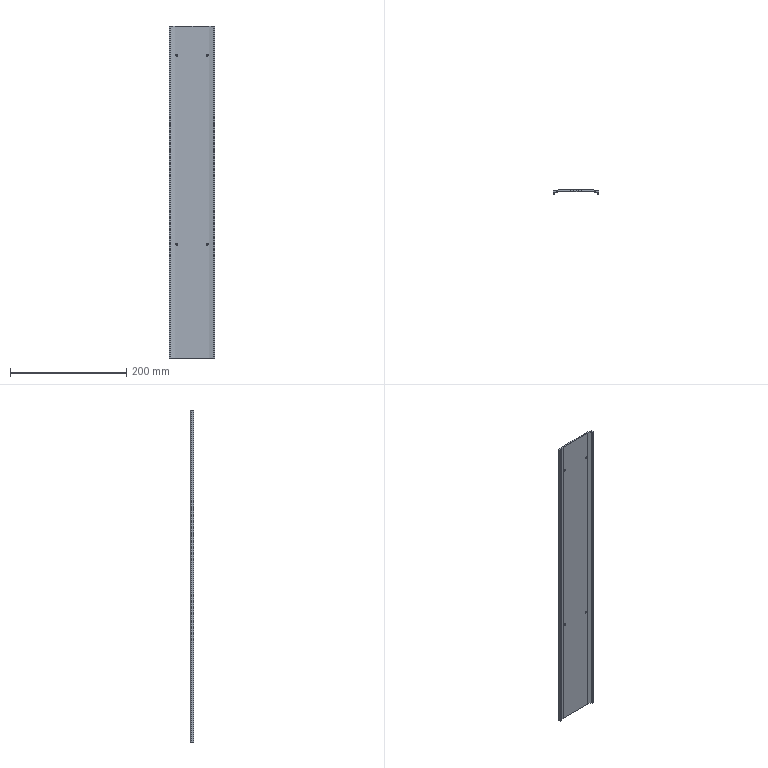Part | NX | 1 solid | 37 faces | box 79 x 6 x 572 mm | volume 116838 mm3 | plane 29 | cylinder 4 | cone 4 | commonest cylinder face diameters 3.4 x4
STEP:
#1=CARTESIAN_POINT('',(518.205,169.433,382.));
#2=VERTEX_POINT('',#1);
#3=CARTESIAN_POINT('',(518.205,165.108,382.));
#4=VERTEX_POINT('',#3);
#5=CARTESIAN_POINT('',(518.205,169.433,382.));
#6=DIRECTION('',(0.,-1.,0.));
#7=VECTOR('',#6,1.);
#8=LINE('',#5,#7);
#9=EDGE_CURVE('',#2,#4,#8,.T.);
#10=ORIENTED_EDGE('',*,*,#9,.F.);
#11=CARTESIAN_POINT('',(518.205,169.433,-190.));
#12=VERTEX_POINT('',#11);
#13=CARTESIAN_POINT('',(518.205,169.433,0.));
#14=DIRECTION('',(0.,0.,1.));
#15=VECTOR('',#14,1.);
#16=LINE('',#13,#15);
#17=EDGE_CURVE('',#12,#2,#16,.T.);
#18=ORIENTED_EDGE('',*,*,#17,.F.);
#19=CARTESIAN_POINT('',(518.205,165.108,-190.));
#20=VERTEX_POINT('',#19);
#21=CARTESIAN_POINT('',(518.205,0.,-190.));
#22=DIRECTION('',(0.,-1.,0.));
#23=VECTOR('',#22,1.);
#24=LINE('',#21,#23);
#25=EDGE_CURVE('',#12,#20,#24,.T.);
#26=ORIENTED_EDGE('',*,*,#25,.T.);
#27=CARTESIAN_POINT('',(518.205,165.108,0.));
#28=DIRECTION('',(0.,0.,1.));
#29=VECTOR('',#28,1.);
#30=LINE('',#27,#29);
#31=EDGE_CURVE('',#20,#4,#30,.T.);
#32=ORIENTED_EDGE('',*,*,#31,.T.);
#33=EDGE_LOOP('',(#10,#18,#26,#32));
#34=FACE_OUTER_BOUND('',#33,.T.);
#35=CARTESIAN_POINT('',(518.205,169.433,0.));
#36=DIRECTION('',(-1.,0.,0.));
#37=DIRECTION('',(0.,0.,-1.));
#38=AXIS2_PLACEMENT_3D('',#35,#36,#37);
#39=PLANE('',#38);
#40=ADVANCED_FACE('',(#34),#39,.T.);
#41=CARTESIAN_POINT('',(520.205,165.108,382.));
#42=VERTEX_POINT('',#41);
#43=CARTESIAN_POINT('',(518.205,165.108,382.));
#44=DIRECTION('',(1.,0.,0.));
#45=VECTOR('',#44,1.);
#46=LINE('',#43,#45);
#47=EDGE_CURVE('',#4,#42,#46,.T.);
#48=ORIENTED_EDGE('',*,*,#47,.F.);
#49=ORIENTED_EDGE('',*,*,#31,.F.);
#50=CARTESIAN_POINT('',(520.205,165.108,-190.));
#51=VERTEX_POINT('',#50);
#52=CARTESIAN_POINT('',(0.,165.108,-190.));
#53=DIRECTION('',(1.,0.,0.));
#54=VECTOR('',#53,1.);
#55=LINE('',#52,#54);
#56=EDGE_CURVE('',#20,#51,#55,.T.);
#57=ORIENTED_EDGE('',*,*,#56,.T.);
#58=CARTESIAN_POINT('',(520.205,165.108,0.));
#59=DIRECTION('',(0.,0.,1.));
#60=VECTOR('',#59,1.);
#61=LINE('',#58,#60);
#62=EDGE_CURVE('',#51,#42,#61,.T.);
#63=ORIENTED_EDGE('',*,*,#62,.T.);
#64=EDGE_LOOP('',(#48,#49,#57,#63));
#65=FACE_OUTER_BOUND('',#64,.T.);
#66=CARTESIAN_POINT('',(518.205,165.108,0.));
#67=DIRECTION('',(0.,-1.,0.));
#68=DIRECTION('',(0.,0.,1.));
#69=AXIS2_PLACEMENT_3D('',#66,#67,#68);
#70=PLANE('',#69);
#71=ADVANCED_FACE('',(#65),#70,.T.);
#72=CARTESIAN_POINT('',(520.205,167.247,382.));
#73=VERTEX_POINT('',#72);
#74=CARTESIAN_POINT('',(520.205,165.108,382.));
#75=DIRECTION('',(0.,1.,0.));
#76=VECTOR('',#75,1.);
#77=LINE('',#74,#76);
#78=EDGE_CURVE('',#42,#73,#77,.T.);
#79=ORIENTED_EDGE('',*,*,#78,.F.);
#80=ORIENTED_EDGE('',*,*,#62,.F.);
#81=CARTESIAN_POINT('',(520.205,167.247,-190.));
#82=VERTEX_POINT('',#81);
#83=CARTESIAN_POINT('',(520.205,0.,-190.));
#84=DIRECTION('',(0.,1.,0.));
#85=VECTOR('',#84,1.);
#86=LINE('',#83,#85);
#87=EDGE_CURVE('',#51,#82,#86,.T.);
#88=ORIENTED_EDGE('',*,*,#87,.T.);
#89=CARTESIAN_POINT('',(520.205,167.247,0.));
#90=DIRECTION('',(0.,0.,1.));
#91=VECTOR('',#90,1.);
#92=LINE('',#89,#91);
#93=EDGE_CURVE('',#82,#73,#92,.T.);
#94=ORIENTED_EDGE('',*,*,#93,.T.);
#95=EDGE_LOOP('',(#79,#80,#88,#94));
#96=FACE_OUTER_BOUND('',#95,.T.);
#97=CARTESIAN_POINT('',(520.205,165.108,0.));
#98=DIRECTION('',(1.,0.,0.));
#99=DIRECTION('',(0.,0.,1.));
#100=AXIS2_PLACEMENT_3D('',#97,#98,#99);
#101=PLANE('',#100);
#102=ADVANCED_FACE('',(#96),#101,.T.);
#103=CARTESIAN_POINT('',(527.924,168.608,382.));
#104=VERTEX_POINT('',#103);
#105=CARTESIAN_POINT('',(520.205,167.247,382.));
#106=DIRECTION('',(0.9848,0.1736,0.));
#107=VECTOR('',#106,1.);
#108=LINE('',#105,#107);
#109=EDGE_CURVE('',#73,#104,#108,.T.);
#110=ORIENTED_EDGE('',*,*,#109,.F.);
#111=ORIENTED_EDGE('',*,*,#93,.F.);
#112=CARTESIAN_POINT('',(527.924,168.608,-190.));
#113=VERTEX_POINT('',#112);
#114=CARTESIAN_POINT('',(-12.915,73.244,-190.));
#115=DIRECTION('',(0.9848,0.1736,0.));
#116=VECTOR('',#115,1.);
#117=LINE('',#114,#116);
#118=EDGE_CURVE('',#82,#113,#117,.T.);
#119=ORIENTED_EDGE('',*,*,#118,.T.);
#120=CARTESIAN_POINT('',(527.924,168.608,0.));
#121=DIRECTION('',(0.,0.,1.));
#122=VECTOR('',#121,1.);
#123=LINE('',#120,#122);
#124=EDGE_CURVE('',#113,#104,#123,.T.);
#125=ORIENTED_EDGE('',*,*,#124,.T.);
#126=EDGE_LOOP('',(#110,#111,#119,#125));
#127=FACE_OUTER_BOUND('',#126,.T.);
#128=CARTESIAN_POINT('',(520.205,167.247,0.));
#129=DIRECTION('',(0.1736,-0.9848,0.));
#130=DIRECTION('',(-0.9848,-0.1736,0.));
#131=AXIS2_PLACEMENT_3D('',#128,#129,#130);
#132=PLANE('',#131);
#133=ADVANCED_FACE('',(#127),#132,.T.);
#134=CARTESIAN_POINT('',(531.705,168.608,329.8));
#135=VERTEX_POINT('',#134);
#136=CARTESIAN_POINT('',(531.705,168.608,331.5));
#137=DIRECTION('',(0.,-1.,0.));
#138=DIRECTION('',(0.,0.,-1.));
#139=AXIS2_PLACEMENT_3D('',#136,#137,#138);
#140=CIRCLE('',#139,1.7);
#141=EDGE_CURVE('',#135,#135,#140,.T.);
#142=ORIENTED_EDGE('',*,*,#141,.F.);
#143=EDGE_LOOP('',(#142));
#144=FACE_BOUND('',#143,.T.);
#145=CARTESIAN_POINT('',(583.705,168.608,4.3));
#146=VERTEX_POINT('',#145);
#147=CARTESIAN_POINT('',(583.705,168.608,6.));
#148=DIRECTION('',(0.,-1.,0.));
#149=DIRECTION('',(0.,0.,-1.));
#150=AXIS2_PLACEMENT_3D('',#147,#148,#149);
#151=CIRCLE('',#150,1.7);
#152=EDGE_CURVE('',#146,#146,#151,.T.);
#153=ORIENTED_EDGE('',*,*,#152,.F.);
#154=EDGE_LOOP('',(#153));
#155=FACE_BOUND('',#154,.T.);
#156=CARTESIAN_POINT('',(583.705,168.608,329.8));
#157=VERTEX_POINT('',#156);
#158=CARTESIAN_POINT('',(583.705,168.608,331.5));
#159=DIRECTION('',(0.,-1.,0.));
#160=DIRECTION('',(0.,0.,-1.));
#161=AXIS2_PLACEMENT_3D('',#158,#159,#160);
#162=CIRCLE('',#161,1.7);
#163=EDGE_CURVE('',#157,#157,#162,.T.);
#164=ORIENTED_EDGE('',*,*,#163,.F.);
#165=EDGE_LOOP('',(#164));
#166=FACE_BOUND('',#165,.T.);
#167=CARTESIAN_POINT('',(531.705,168.608,4.3));
#168=VERTEX_POINT('',#167);
#169=CARTESIAN_POINT('',(531.705,168.608,6.));
#170=DIRECTION('',(0.,-1.,0.));
#171=DIRECTION('',(0.,0.,-1.));
#172=AXIS2_PLACEMENT_3D('',#169,#170,#171);
#173=CIRCLE('',#172,1.7);
#174=EDGE_CURVE('',#168,#168,#173,.T.);
#175=ORIENTED_EDGE('',*,*,#174,.F.);
#176=EDGE_LOOP('',(#175));
#177=FACE_BOUND('',#176,.T.);
#178=CARTESIAN_POINT('',(587.487,168.608,382.));
#179=VERTEX_POINT('',#178);
#180=CARTESIAN_POINT('',(527.924,168.608,382.));
#181=DIRECTION('',(1.,0.,0.));
#182=VECTOR('',#181,1.);
#183=LINE('',#180,#182);
#184=EDGE_CURVE('',#104,#179,#183,.T.);
#185=ORIENTED_EDGE('',*,*,#184,.F.);
#186=ORIENTED_EDGE('',*,*,#124,.F.);
#187=CARTESIAN_POINT('',(587.487,168.608,-190.));
#188=VERTEX_POINT('',#187);
#189=CARTESIAN_POINT('',(0.,168.608,-190.));
#190=DIRECTION('',(1.,0.,0.));
#191=VECTOR('',#190,1.);
#192=LINE('',#189,#191);
#193=EDGE_CURVE('',#113,#188,#192,.T.);
#194=ORIENTED_EDGE('',*,*,#193,.T.);
#195=CARTESIAN_POINT('',(587.487,168.608,0.));
#196=DIRECTION('',(0.,0.,1.));
#197=VECTOR('',#196,1.);
#198=LINE('',#195,#197);
#199=EDGE_CURVE('',#188,#179,#198,.T.);
#200=ORIENTED_EDGE('',*,*,#199,.T.);
#201=EDGE_LOOP('',(#185,#186,#194,#200));
#202=FACE_BOUND('',#201,.T.);
#203=CARTESIAN_POINT('',(527.924,168.608,0.));
#204=DIRECTION('',(0.,-1.,0.));
#205=DIRECTION('',(0.,0.,1.));
#206=AXIS2_PLACEMENT_3D('',#203,#204,#205);
#207=PLANE('',#206);
#208=ADVANCED_FACE('',(#144,#155,#166,#177,#202),#207,.T.);
#209=CARTESIAN_POINT('',(595.205,167.247,382.));
#210=VERTEX_POINT('',#209);
#211=CARTESIAN_POINT('',(587.487,168.608,382.));
#212=DIRECTION('',(0.9848,-0.1736,0.));
#213=VECTOR('',#212,1.);
#214=LINE('',#211,#213);
#215=EDGE_CURVE('',#179,#210,#214,.T.);
#216=ORIENTED_EDGE('',*,*,#215,.F.);
#217=ORIENTED_EDGE('',*,*,#199,.F.);
#218=CARTESIAN_POINT('',(595.205,167.247,-190.));
#219=VERTEX_POINT('',#218);
#220=CARTESIAN_POINT('',(46.549,263.99,-190.));
#221=DIRECTION('',(0.9848,-0.1736,0.));
#222=VECTOR('',#221,1.);
#223=LINE('',#220,#222);
#224=EDGE_CURVE('',#188,#219,#223,.T.);
#225=ORIENTED_EDGE('',*,*,#224,.T.);
#226=CARTESIAN_POINT('',(595.205,167.247,0.));
#227=DIRECTION('',(0.,0.,1.));
#228=VECTOR('',#227,1.);
#229=LINE('',#226,#228);
#230=EDGE_CURVE('',#219,#210,#229,.T.);
#231=ORIENTED_EDGE('',*,*,#230,.T.);
#232=EDGE_LOOP('',(#216,#217,#225,#231));
#233=FACE_OUTER_BOUND('',#232,.T.);
#234=CARTESIAN_POINT('',(587.487,168.608,0.));
#235=DIRECTION('',(-0.1736,-0.9848,0.));
#236=DIRECTION('',(-0.9848,0.1736,0.));
#237=AXIS2_PLACEMENT_3D('',#234,#235,#236);
#238=PLANE('',#237);
#239=ADVANCED_FACE('',(#233),#238,.T.);
#240=CARTESIAN_POINT('',(595.205,165.108,382.));
#241=VERTEX_POINT('',#240);
#242=CARTESIAN_POINT('',(595.205,167.247,382.));
#243=DIRECTION('',(0.,-1.,0.));
#244=VECTOR('',#243,1.);
#245=LINE('',#242,#244);
#246=EDGE_CURVE('',#210,#241,#245,.T.);
#247=ORIENTED_EDGE('',*,*,#246,.F.);
#248=ORIENTED_EDGE('',*,*,#230,.F.);
#249=CARTESIAN_POINT('',(595.205,165.108,-190.));
#250=VERTEX_POINT('',#249);
#251=CARTESIAN_POINT('',(595.205,0.,-190.));
#252=DIRECTION('',(0.,-1.,0.));
#253=VECTOR('',#252,1.);
#254=LINE('',#251,#253);
#255=EDGE_CURVE('',#219,#250,#254,.T.);
#256=ORIENTED_EDGE('',*,*,#255,.T.);
#257=CARTESIAN_POINT('',(595.205,165.108,0.));
#258=DIRECTION('',(0.,0.,1.));
#259=VECTOR('',#258,1.);
#260=LINE('',#257,#259);
#261=EDGE_CURVE('',#250,#241,#260,.T.);
#262=ORIENTED_EDGE('',*,*,#261,.T.);
#263=EDGE_LOOP('',(#247,#248,#256,#262));
#264=FACE_OUTER_BOUND('',#263,.T.);
#265=CARTESIAN_POINT('',(595.205,167.247,0.));
#266=DIRECTION('',(-1.,0.,0.));
#267=DIRECTION('',(0.,0.,-1.));
#268=AXIS2_PLACEMENT_3D('',#265,#266,#267);
#269=PLANE('',#268);
#270=ADVANCED_FACE('',(#264),#269,.T.);
#271=CARTESIAN_POINT('',(597.205,165.108,382.));
#272=VERTEX_POINT('',#271);
#273=CARTESIAN_POINT('',(595.205,165.108,382.));
#274=DIRECTION('',(1.,0.,0.));
#275=VECTOR('',#274,1.);
#276=LINE('',#273,#275);
#277=EDGE_CURVE('',#241,#272,#276,.T.);
#278=ORIENTED_EDGE('',*,*,#277,.F.);
#279=ORIENTED_EDGE('',*,*,#261,.F.);
#280=CARTESIAN_POINT('',(597.205,165.108,-190.));
#281=VERTEX_POINT('',#280);
#282=CARTESIAN_POINT('',(0.,165.108,-190.));
#283=DIRECTION('',(1.,0.,0.));
#284=VECTOR('',#283,1.);
#285=LINE('',#282,#284);
#286=EDGE_CURVE('',#250,#281,#285,.T.);
#287=ORIENTED_EDGE('',*,*,#286,.T.);
#288=CARTESIAN_POINT('',(597.205,165.108,0.));
#289=DIRECTION('',(0.,0.,1.));
#290=VECTOR('',#289,1.);
#291=LINE('',#288,#290);
#292=EDGE_CURVE('',#281,#272,#291,.T.);
#293=ORIENTED_EDGE('',*,*,#292,.T.);
#294=EDGE_LOOP('',(#278,#279,#287,#293));
#295=FACE_OUTER_BOUND('',#294,.T.);
#296=CARTESIAN_POINT('',(595.205,165.108,0.));
#297=DIRECTION('',(0.,-1.,0.));
#298=DIRECTION('',(0.,0.,1.));
#299=AXIS2_PLACEMENT_3D('',#296,#297,#298);
#300=PLANE('',#299);
#301=ADVANCED_FACE('',(#295),#300,.T.);
#302=CARTESIAN_POINT('',(597.205,169.433,382.));
#303=VERTEX_POINT('',#302);
#304=CARTESIAN_POINT('',(597.205,165.108,382.));
#305=DIRECTION('',(0.,1.,0.));
#306=VECTOR('',#305,1.);
#307=LINE('',#304,#306);
#308=EDGE_CURVE('',#272,#303,#307,.T.);
#309=ORIENTED_EDGE('',*,*,#308,.F.);
#310=ORIENTED_EDGE('',*,*,#292,.F.);
#311=CARTESIAN_POINT('',(597.205,169.433,-190.));
#312=VERTEX_POINT('',#311);
#313=CARTESIAN_POINT('',(597.205,0.,-190.));
#314=DIRECTION('',(0.,1.,0.));
#315=VECTOR('',#314,1.);
#316=LINE('',#313,#315);
#317=EDGE_CURVE('',#281,#312,#316,.T.);
#318=ORIENTED_EDGE('',*,*,#317,.T.);
#319=CARTESIAN_POINT('',(597.205,169.433,0.));
#320=DIRECTION('',(0.,0.,1.));
#321=VECTOR('',#320,1.);
#322=LINE('',#319,#321);
#323=EDGE_CURVE('',#312,#303,#322,.T.);
#324=ORIENTED_EDGE('',*,*,#323,.T.);
#325=EDGE_LOOP('',(#309,#310,#318,#324));
#326=FACE_OUTER_BOUND('',#325,.T.);
#327=CARTESIAN_POINT('',(597.205,165.108,0.));
#328=DIRECTION('',(1.,0.,0.));
#329=DIRECTION('',(0.,0.,1.));
#330=AXIS2_PLACEMENT_3D('',#327,#328,#329);
#331=PLANE('',#330);
#332=ADVANCED_FACE('',(#326),#331,.T.);
#333=CARTESIAN_POINT('',(587.705,171.108,382.));
#334=VERTEX_POINT('',#333);
#335=CARTESIAN_POINT('',(597.205,169.433,382.));
#336=DIRECTION('',(-0.9848,0.1736,0.));
#337=VECTOR('',#336,1.);
#338=LINE('',#335,#337);
#339=EDGE_CURVE('',#303,#334,#338,.T.);
#340=ORIENTED_EDGE('',*,*,#339,.F.);
#341=ORIENTED_EDGE('',*,*,#323,.F.);
#342=CARTESIAN_POINT('',(587.705,171.108,-190.));
#343=VERTEX_POINT('',#342);
#344=CARTESIAN_POINT('',(46.983,266.452,-190.));
#345=DIRECTION('',(-0.9848,0.1736,0.));
#346=VECTOR('',#345,1.);
#347=LINE('',#344,#346);
#348=EDGE_CURVE('',#312,#343,#347,.T.);
#349=ORIENTED_EDGE('',*,*,#348,.T.);
#350=CARTESIAN_POINT('',(587.705,171.108,0.));
#351=DIRECTION('',(0.,0.,1.));
#352=VECTOR('',#351,1.);
#353=LINE('',#350,#352);
#354=EDGE_CURVE('',#343,#334,#353,.T.);
#355=ORIENTED_EDGE('',*,*,#354,.T.);
#356=EDGE_LOOP('',(#340,#341,#349,#355));
#357=FACE_OUTER_BOUND('',#356,.T.);
#358=CARTESIAN_POINT('',(597.205,169.433,0.));
#359=DIRECTION('',(0.1736,0.9848,0.));
#360=DIRECTION('',(0.9848,-0.1736,0.));
#361=AXIS2_PLACEMENT_3D('',#358,#359,#360);
#362=PLANE('',#361);
#363=ADVANCED_FACE('',(#357),#362,.T.);
#364=CARTESIAN_POINT('',(583.705,171.108,9.3));
#365=VERTEX_POINT('',#364);
#366=CARTESIAN_POINT('',(583.705,171.108,6.));
#367=DIRECTION('',(0.,-1.,0.));
#368=DIRECTION('',(0.,0.,1.));
#369=AXIS2_PLACEMENT_3D('',#366,#367,#368);
#370=CIRCLE('',#369,3.3);
#371=EDGE_CURVE('',#365,#365,#370,.T.);
#372=ORIENTED_EDGE('',*,*,#371,.T.);
#373=EDGE_LOOP('',(#372));
#374=FACE_BOUND('',#373,.T.);
#375=CARTESIAN_POINT('',(583.705,171.108,334.8));
#376=VERTEX_POINT('',#375);
#377=CARTESIAN_POINT('',(583.705,171.108,331.5));
#378=DIRECTION('',(0.,-1.,0.));
#379=DIRECTION('',(0.,0.,1.));
#380=AXIS2_PLACEMENT_3D('',#377,#378,#379);
#381=CIRCLE('',#380,3.3);
#382=EDGE_CURVE('',#376,#376,#381,.T.);
#383=ORIENTED_EDGE('',*,*,#382,.T.);
#384=EDGE_LOOP('',(#383));
#385=FACE_BOUND('',#384,.T.);
#386=CARTESIAN_POINT('',(568.323,171.108,382.));
#387=VERTEX_POINT('',#386);
#388=CARTESIAN_POINT('',(587.705,171.108,382.));
#389=DIRECTION('',(-1.,0.,0.));
#390=VECTOR('',#389,1.);
#391=LINE('',#388,#390);
#392=EDGE_CURVE('',#334,#387,#391,.T.);
#393=ORIENTED_EDGE('',*,*,#392,.F.);
#394=ORIENTED_EDGE('',*,*,#354,.F.);
#395=CARTESIAN_POINT('',(568.323,171.108,-190.));
#396=VERTEX_POINT('',#395);
#397=CARTESIAN_POINT('',(0.,171.108,-190.));
#398=DIRECTION('',(-1.,0.,0.));
#399=VECTOR('',#398,1.);
#400=LINE('',#397,#399);
#401=EDGE_CURVE('',#343,#396,#400,.T.);
#402=ORIENTED_EDGE('',*,*,#401,.T.);
#403=CARTESIAN_POINT('',(568.323,171.108,0.));
#404=DIRECTION('',(0.,0.,1.));
#405=VECTOR('',#404,1.);
#406=LINE('',#403,#405);
#407=EDGE_CURVE('',#396,#387,#406,.T.);
#408=ORIENTED_EDGE('',*,*,#407,.T.);
#409=EDGE_LOOP('',(#393,#394,#402,#408));
#410=FACE_BOUND('',#409,.T.);
#411=CARTESIAN_POINT('',(587.705,171.108,0.));
#412=DIRECTION('',(0.,1.,0.));
#413=DIRECTION('',(0.,0.,-1.));
#414=AXIS2_PLACEMENT_3D('',#411,#412,#413);
#415=PLANE('',#414);
#416=ADVANCED_FACE('',(#374,#385,#410),#415,.T.);
#417=CARTESIAN_POINT('',(567.705,170.608,382.));
#418=VERTEX_POINT('',#417);
#419=CARTESIAN_POINT('',(568.323,171.108,382.));
#420=DIRECTION('',(-0.7774,-0.629,0.));
#421=VECTOR('',#420,1.);
#422=LINE('',#419,#421);
#423=EDGE_CURVE('',#387,#418,#422,.T.);
#424=ORIENTED_EDGE('',*,*,#423,.F.);
#425=ORIENTED_EDGE('',*,*,#407,.F.);
#426=CARTESIAN_POINT('',(567.705,170.608,-190.));
#427=VERTEX_POINT('',#426);
#428=CARTESIAN_POINT('',(141.154,-174.477,-190.));
#429=DIRECTION('',(-0.7774,-0.629,0.));
#430=VECTOR('',#429,1.);
#431=LINE('',#428,#430);
#432=EDGE_CURVE('',#396,#427,#431,.T.);
#433=ORIENTED_EDGE('',*,*,#432,.T.);
#434=CARTESIAN_POINT('',(567.705,170.608,0.));
#435=DIRECTION('',(0.,0.,1.));
#436=VECTOR('',#435,1.);
#437=LINE('',#434,#436);
#438=EDGE_CURVE('',#427,#418,#437,.T.);
#439=ORIENTED_EDGE('',*,*,#438,.T.);
#440=EDGE_LOOP('',(#424,#425,#433,#439));
#441=FACE_OUTER_BOUND('',#440,.T.);
#442=CARTESIAN_POINT('',(568.323,171.108,0.));
#443=DIRECTION('',(-0.629,0.7774,0.));
#444=DIRECTION('',(0.7774,0.629,0.));
#445=AXIS2_PLACEMENT_3D('',#442,#443,#444);
#446=PLANE('',#445);
#447=ADVANCED_FACE('',(#441),#446,.T.);
#448=CARTESIAN_POINT('',(567.087,171.108,382.));
#449=VERTEX_POINT('',#448);
#450=CARTESIAN_POINT('',(567.705,170.608,382.));
#451=DIRECTION('',(-0.7774,0.629,0.));
#452=VECTOR('',#451,1.);
#453=LINE('',#450,#452);
#454=EDGE_CURVE('',#418,#449,#453,.T.);
#455=ORIENTED_EDGE('',*,*,#454,.F.);
#456=ORIENTED_EDGE('',*,*,#438,.F.);
#457=CARTESIAN_POINT('',(567.087,171.108,-190.));
#458=VERTEX_POINT('',#457);
#459=CARTESIAN_POINT('',(308.001,380.712,-190.));
#460=DIRECTION('',(-0.7774,0.629,0.));
#461=VECTOR('',#460,1.);
#462=LINE('',#459,#461);
#463=EDGE_CURVE('',#427,#458,#462,.T.);
#464=ORIENTED_EDGE('',*,*,#463,.T.);
#465=CARTESIAN_POINT('',(567.087,171.108,0.));
#466=DIRECTION('',(0.,0.,1.));
#467=VECTOR('',#466,1.);
#468=LINE('',#465,#467);
#469=EDGE_CURVE('',#458,#449,#468,.T.);
#470=ORIENTED_EDGE('',*,*,#469,.T.);
#471=EDGE_LOOP('',(#455,#456,#464,#470));
#472=FACE_OUTER_BOUND('',#471,.T.);
#473=CARTESIAN_POINT('',(567.705,170.608,0.));
#474=DIRECTION('',(0.629,0.7774,0.));
#475=DIRECTION('',(0.7774,-0.629,0.));
#476=AXIS2_PLACEMENT_3D('',#473,#474,#475);
#477=PLANE('',#476);
#478=ADVANCED_FACE('',(#472),#477,.T.);
#479=CARTESIAN_POINT('',(563.323,171.108,382.));
#480=VERTEX_POINT('',#479);
#481=CARTESIAN_POINT('',(567.087,171.108,382.));
#482=DIRECTION('',(-1.,0.,0.));
#483=VECTOR('',#482,1.);
#484=LINE('',#481,#483);
#485=EDGE_CURVE('',#449,#480,#484,.T.);
#486=ORIENTED_EDGE('',*,*,#485,.F.);
#487=ORIENTED_EDGE('',*,*,#469,.F.);
#488=CARTESIAN_POINT('',(563.323,171.108,-190.));
#489=VERTEX_POINT('',#488);
#490=CARTESIAN_POINT('',(0.,171.108,-190.));
#491=DIRECTION('',(-1.,0.,0.));
#492=VECTOR('',#491,1.);
#493=LINE('',#490,#492);
#494=EDGE_CURVE('',#458,#489,#493,.T.);
#495=ORIENTED_EDGE('',*,*,#494,.T.);
#496=CARTESIAN_POINT('',(563.323,171.108,0.));
#497=DIRECTION('',(0.,0.,1.));
#498=VECTOR('',#497,1.);
#499=LINE('',#496,#498);
#500=EDGE_CURVE('',#489,#480,#499,.T.);
#501=ORIENTED_EDGE('',*,*,#500,.T.);
#502=EDGE_LOOP('',(#486,#487,#495,#501));
#503=FACE_OUTER_BOUND('',#502,.T.);
#504=CARTESIAN_POINT('',(567.087,171.108,0.));
#505=DIRECTION('',(0.,1.,0.));
#506=DIRECTION('',(0.,0.,-1.));
#507=AXIS2_PLACEMENT_3D('',#504,#505,#506);
#508=PLANE('',#507);
#509=ADVANCED_FACE('',(#503),#508,.T.);
#510=CARTESIAN_POINT('',(562.705,170.608,382.));
#511=VERTEX_POINT('',#510);
#512=CARTESIAN_POINT('',(563.323,171.108,382.));
#513=DIRECTION('',(-0.7774,-0.629,0.));
#514=VECTOR('',#513,1.);
#515=LINE('',#512,#514);
#516=EDGE_CURVE('',#480,#511,#515,.T.);
#517=ORIENTED_EDGE('',*,*,#516,.F.);
#518=ORIENTED_EDGE('',*,*,#500,.F.);
#519=CARTESIAN_POINT('',(562.705,170.608,-190.));
#520=VERTEX_POINT('',#519);
#521=CARTESIAN_POINT('',(139.176,-172.032,-190.));
#522=DIRECTION('',(-0.7774,-0.629,0.));
#523=VECTOR('',#522,1.);
#524=LINE('',#521,#523);
#525=EDGE_CURVE('',#489,#520,#524,.T.);
#526=ORIENTED_EDGE('',*,*,#525,.T.);
#527=CARTESIAN_POINT('',(562.705,170.608,0.));
#528=DIRECTION('',(0.,0.,1.));
#529=VECTOR('',#528,1.);
#530=LINE('',#527,#529);
#531=EDGE_CURVE('',#520,#511,#530,.T.);
#532=ORIENTED_EDGE('',*,*,#531,.T.);
#533=EDGE_LOOP('',(#517,#518,#526,#532));
#534=FACE_OUTER_BOUND('',#533,.T.);
#535=CARTESIAN_POINT('',(563.323,171.108,0.));
#536=DIRECTION('',(-0.629,0.7774,0.));
#537=DIRECTION('',(0.7774,0.629,0.));
#538=AXIS2_PLACEMENT_3D('',#535,#536,#537);
#539=PLANE('',#538);
#540=ADVANCED_FACE('',(#534),#539,.T.);
#541=CARTESIAN_POINT('',(562.087,171.108,382.));
#542=VERTEX_POINT('',#541);
#543=CARTESIAN_POINT('',(562.705,170.608,382.));
#544=DIRECTION('',(-0.7774,0.629,0.));
#545=VECTOR('',#544,1.);
#546=LINE('',#543,#545);
#547=EDGE_CURVE('',#511,#542,#546,.T.);
#548=ORIENTED_EDGE('',*,*,#547,.F.);
#549=ORIENTED_EDGE('',*,*,#531,.F.);
#550=CARTESIAN_POINT('',(562.087,171.108,-190.));
#551=VERTEX_POINT('',#550);
#552=CARTESIAN_POINT('',(306.023,378.267,-190.));
#553=DIRECTION('',(-0.7774,0.629,0.));
#554=VECTOR('',#553,1.);
#555=LINE('',#552,#554);
#556=EDGE_CURVE('',#520,#551,#555,.T.);
#557=ORIENTED_EDGE('',*,*,#556,.T.);
#558=CARTESIAN_POINT('',(562.087,171.108,0.));
#559=DIRECTION('',(0.,0.,1.));
#560=VECTOR('',#559,1.);
#561=LINE('',#558,#560);
#562=EDGE_CURVE('',#551,#542,#561,.T.);
#563=ORIENTED_EDGE('',*,*,#562,.T.);
#564=EDGE_LOOP('',(#548,#549,#557,#563));
#565=FACE_OUTER_BOUND('',#564,.T.);
#566=CARTESIAN_POINT('',(562.705,170.608,0.));
#567=DIRECTION('',(0.629,0.7774,0.));
#568=DIRECTION('',(0.7774,-0.629,0.));
#569=AXIS2_PLACEMENT_3D('',#566,#567,#568);
#570=PLANE('',#569);
#571=ADVANCED_FACE('',(#565),#570,.T.);
#572=CARTESIAN_POINT('',(558.323,171.108,382.));
#573=VERTEX_POINT('',#572);
#574=CARTESIAN_POINT('',(562.087,171.108,382.));
#575=DIRECTION('',(-1.,0.,0.));
#576=VECTOR('',#575,1.);
#577=LINE('',#574,#576);
#578=EDGE_CURVE('',#542,#573,#577,.T.);
#579=ORIENTED_EDGE('',*,*,#578,.F.);
#580=ORIENTED_EDGE('',*,*,#562,.F.);
#581=CARTESIAN_POINT('',(558.323,171.108,-190.));
#582=VERTEX_POINT('',#581);
#583=CARTESIAN_POINT('',(0.,171.108,-190.));
#584=DIRECTION('',(-1.,0.,0.));
#585=VECTOR('',#584,1.);
#586=LINE('',#583,#585);
#587=EDGE_CURVE('',#551,#582,#586,.T.);
#588=ORIENTED_EDGE('',*,*,#587,.T.);
#589=CARTESIAN_POINT('',(558.323,171.108,0.));
#590=DIRECTION('',(0.,0.,1.));
#591=VECTOR('',#590,1.);
#592=LINE('',#589,#591);
#593=EDGE_CURVE('',#582,#573,#592,.T.);
#594=ORIENTED_EDGE('',*,*,#593,.T.);
#595=EDGE_LOOP('',(#579,#580,#588,#594));
#596=FACE_OUTER_BOUND('',#595,.T.);
#597=CARTESIAN_POINT('',(562.087,171.108,0.));
#598=DIRECTION('',(0.,1.,0.));
#599=DIRECTION('',(0.,0.,-1.));
#600=AXIS2_PLACEMENT_3D('',#597,#598,#599);
#601=PLANE('',#600);
#602=ADVANCED_FACE('',(#596),#601,.T.);
#603=CARTESIAN_POINT('',(557.705,170.608,382.));
#604=VERTEX_POINT('',#603);
#605=CARTESIAN_POINT('',(558.323,171.108,382.));
#606=DIRECTION('',(-0.7774,-0.629,0.));
#607=VECTOR('',#606,1.);
#608=LINE('',#605,#607);
#609=EDGE_CURVE('',#573,#604,#608,.T.);
#610=ORIENTED_EDGE('',*,*,#609,.F.);
#611=ORIENTED_EDGE('',*,*,#593,.F.);
#612=CARTESIAN_POINT('',(557.705,170.608,-190.));
#613=VERTEX_POINT('',#612);
#614=CARTESIAN_POINT('',(137.199,-169.588,-190.));
#615=DIRECTION('',(-0.7774,-0.629,0.));
#616=VECTOR('',#615,1.);
#617=LINE('',#614,#616);
#618=EDGE_CURVE('',#582,#613,#617,.T.);
#619=ORIENTED_EDGE('',*,*,#618,.T.);
#620=CARTESIAN_POINT('',(557.705,170.608,0.));
#621=DIRECTION('',(0.,0.,1.));
#622=VECTOR('',#621,1.);
#623=LINE('',#620,#622);
#624=EDGE_CURVE('',#613,#604,#623,.T.);
#625=ORIENTED_EDGE('',*,*,#624,.T.);
#626=EDGE_LOOP('',(#610,#611,#619,#625));
#627=FACE_OUTER_BOUND('',#626,.T.);
#628=CARTESIAN_POINT('',(558.323,171.108,0.));
#629=DIRECTION('',(-0.629,0.7774,0.));
#630=DIRECTION('',(0.7774,0.629,0.));
#631=AXIS2_PLACEMENT_3D('',#628,#629,#630);
#632=PLANE('',#631);
#633=ADVANCED_FACE('',(#627),#632,.T.);
#634=CARTESIAN_POINT('',(557.087,171.108,382.));
#635=VERTEX_POINT('',#634);
#636=CARTESIAN_POINT('',(557.705,170.608,382.));
#637=DIRECTION('',(-0.7774,0.629,0.));
#638=VECTOR('',#637,1.);
#639=LINE('',#636,#638);
#640=EDGE_CURVE('',#604,#635,#639,.T.);
#641=ORIENTED_EDGE('',*,*,#640,.F.);
#642=ORIENTED_EDGE('',*,*,#624,.F.);
#643=CARTESIAN_POINT('',(557.087,171.108,-190.));
#644=VERTEX_POINT('',#643);
#645=CARTESIAN_POINT('',(304.045,375.822,-190.));
#646=DIRECTION('',(-0.7774,0.629,0.));
#647=VECTOR('',#646,1.);
#648=LINE('',#645,#647);
#649=EDGE_CURVE('',#613,#644,#648,.T.);
#650=ORIENTED_EDGE('',*,*,#649,.T.);
#651=CARTESIAN_POINT('',(557.087,171.108,0.));
#652=DIRECTION('',(0.,0.,1.));
#653=VECTOR('',#652,1.);
#654=LINE('',#651,#653);
#655=EDGE_CURVE('',#644,#635,#654,.T.);
#656=ORIENTED_EDGE('',*,*,#655,.T.);
#657=EDGE_LOOP('',(#641,#642,#650,#656));
#658=FACE_OUTER_BOUND('',#657,.T.);
#659=CARTESIAN_POINT('',(557.705,170.608,0.));
#660=DIRECTION('',(0.629,0.7774,0.));
#661=DIRECTION('',(0.7774,-0.629,0.));
#662=AXIS2_PLACEMENT_3D('',#659,#660,#661);
#663=PLANE('',#662);
#664=ADVANCED_FACE('',(#658),#663,.T.);
#665=CARTESIAN_POINT('',(553.323,171.108,382.));
#666=VERTEX_POINT('',#665);
#667=CARTESIAN_POINT('',(557.087,171.108,382.));
#668=DIRECTION('',(-1.,0.,0.));
#669=VECTOR('',#668,1.);
#670=LINE('',#667,#669);
#671=EDGE_CURVE('',#635,#666,#670,.T.);
#672=ORIENTED_EDGE('',*,*,#671,.F.);
#673=ORIENTED_EDGE('',*,*,#655,.F.);
#674=CARTESIAN_POINT('',(553.323,171.108,-190.));
#675=VERTEX_POINT('',#674);
#676=CARTESIAN_POINT('',(0.,171.108,-190.));
#677=DIRECTION('',(-1.,0.,0.));
#678=VECTOR('',#677,1.);
#679=LINE('',#676,#678);
#680=EDGE_CURVE('',#644,#675,#679,.T.);
#681=ORIENTED_EDGE('',*,*,#680,.T.);
#682=CARTESIAN_POINT('',(553.323,171.108,0.));
#683=DIRECTION('',(0.,0.,1.));
#684=VECTOR('',#683,1.);
#685=LINE('',#682,#684);
#686=EDGE_CURVE('',#675,#666,#685,.T.);
#687=ORIENTED_EDGE('',*,*,#686,.T.);
#688=EDGE_LOOP('',(#672,#673,#681,#687));
#689=FACE_OUTER_BOUND('',#688,.T.);
#690=CARTESIAN_POINT('',(557.087,171.108,0.));
#691=DIRECTION('',(0.,1.,0.));
#692=DIRECTION('',(0.,0.,-1.));
#693=AXIS2_PLACEMENT_3D('',#690,#691,#692);
#694=PLANE('',#693);
#695=ADVANCED_FACE('',(#689),#694,.T.);
#696=CARTESIAN_POINT('',(552.705,170.608,382.));
#697=VERTEX_POINT('',#696);
#698=CARTESIAN_POINT('',(553.323,171.108,382.));
#699=DIRECTION('',(-0.7774,-0.629,0.));
#700=VECTOR('',#699,1.);
#701=LINE('',#698,#700);
#702=EDGE_CURVE('',#666,#697,#701,.T.);
#703=ORIENTED_EDGE('',*,*,#702,.F.);
#704=ORIENTED_EDGE('',*,*,#686,.F.);
#705=CARTESIAN_POINT('',(552.705,170.608,-190.));
#706=VERTEX_POINT('',#705);
#707=CARTESIAN_POINT('',(135.221,-167.143,-190.));
#708=DIRECTION('',(-0.7774,-0.629,0.));
#709=VECTOR('',#708,1.);
#710=LINE('',#707,#709);
#711=EDGE_CURVE('',#675,#706,#710,.T.);
#712=ORIENTED_EDGE('',*,*,#711,.T.);
#713=CARTESIAN_POINT('',(552.705,170.608,0.));
#714=DIRECTION('',(0.,0.,1.));
#715=VECTOR('',#714,1.);
#716=LINE('',#713,#715);
#717=EDGE_CURVE('',#706,#697,#716,.T.);
#718=ORIENTED_EDGE('',*,*,#717,.T.);
#719=EDGE_LOOP('',(#703,#704,#712,#718));
#720=FACE_OUTER_BOUND('',#719,.T.);
#721=CARTESIAN_POINT('',(553.323,171.108,0.));
#722=DIRECTION('',(-0.629,0.7774,0.));
#723=DIRECTION('',(0.7774,0.629,0.));
#724=AXIS2_PLACEMENT_3D('',#721,#722,#723);
#725=PLANE('',#724);
#726=ADVANCED_FACE('',(#720),#725,.T.);
#727=CARTESIAN_POINT('',(552.087,171.108,382.));
#728=VERTEX_POINT('',#727);
#729=CARTESIAN_POINT('',(552.705,170.608,382.));
#730=DIRECTION('',(-0.7774,0.629,0.));
#731=VECTOR('',#730,1.);
#732=LINE('',#729,#731);
#733=EDGE_CURVE('',#697,#728,#732,.T.);
#734=ORIENTED_EDGE('',*,*,#733,.F.);
#735=ORIENTED_EDGE('',*,*,#717,.F.);
#736=CARTESIAN_POINT('',(552.087,171.108,-190.));
#737=VERTEX_POINT('',#736);
#738=CARTESIAN_POINT('',(302.067,373.378,-190.));
#739=DIRECTION('',(-0.7774,0.629,0.));
#740=VECTOR('',#739,1.);
#741=LINE('',#738,#740);
#742=EDGE_CURVE('',#706,#737,#741,.T.);
#743=ORIENTED_EDGE('',*,*,#742,.T.);
#744=CARTESIAN_POINT('',(552.087,171.108,0.));
#745=DIRECTION('',(0.,0.,1.));
#746=VECTOR('',#745,1.);
#747=LINE('',#744,#746);
#748=EDGE_CURVE('',#737,#728,#747,.T.);
#749=ORIENTED_EDGE('',*,*,#748,.T.);
#750=EDGE_LOOP('',(#734,#735,#743,#749));
#751=FACE_OUTER_BOUND('',#750,.T.);
#752=CARTESIAN_POINT('',(552.705,170.608,0.));
#753=DIRECTION('',(0.629,0.7774,0.));
#754=DIRECTION('',(0.7774,-0.629,0.));
#755=AXIS2_PLACEMENT_3D('',#752,#753,#754);
#756=PLANE('',#755);
#757=ADVANCED_FACE('',(#751),#756,.T.);
#758=CARTESIAN_POINT('',(548.323,171.108,382.));
#759=VERTEX_POINT('',#758);
#760=CARTESIAN_POINT('',(552.087,171.108,382.));
#761=DIRECTION('',(-1.,0.,0.));
#762=VECTOR('',#761,1.);
#763=LINE('',#760,#762);
#764=EDGE_CURVE('',#728,#759,#763,.T.);
#765=ORIENTED_EDGE('',*,*,#764,.F.);
#766=ORIENTED_EDGE('',*,*,#748,.F.);
#767=CARTESIAN_POINT('',(548.323,171.108,-190.));
#768=VERTEX_POINT('',#767);
#769=CARTESIAN_POINT('',(0.,171.108,-190.));
#770=DIRECTION('',(-1.,0.,0.));
#771=VECTOR('',#770,1.);
#772=LINE('',#769,#771);
#773=EDGE_CURVE('',#737,#768,#772,.T.);
#774=ORIENTED_EDGE('',*,*,#773,.T.);
#775=CARTESIAN_POINT('',(548.323,171.108,0.));
#776=DIRECTION('',(0.,0.,1.));
#777=VECTOR('',#776,1.);
#778=LINE('',#775,#777);
#779=EDGE_CURVE('',#768,#759,#778,.T.);
#780=ORIENTED_EDGE('',*,*,#779,.T.);
#781=EDGE_LOOP('',(#765,#766,#774,#780));
#782=FACE_OUTER_BOUND('',#781,.T.);
#783=CARTESIAN_POINT('',(552.087,171.108,0.));
#784=DIRECTION('',(0.,1.,0.));
#785=DIRECTION('',(0.,0.,-1.));
#786=AXIS2_PLACEMENT_3D('',#783,#784,#785);
#787=PLANE('',#786);
#788=ADVANCED_FACE('',(#782),#787,.T.);
#789=CARTESIAN_POINT('',(547.705,170.608,382.));
#790=VERTEX_POINT('',#789);
#791=CARTESIAN_POINT('',(548.323,171.108,382.));
#792=DIRECTION('',(-0.7774,-0.629,0.));
#793=VECTOR('',#792,1.);
#794=LINE('',#791,#793);
#795=EDGE_CURVE('',#759,#790,#794,.T.);
#796=ORIENTED_EDGE('',*,*,#795,.F.);
#797=ORIENTED_EDGE('',*,*,#779,.F.);
#798=CARTESIAN_POINT('',(547.705,170.608,-190.));
#799=VERTEX_POINT('',#798);
#800=CARTESIAN_POINT('',(133.243,-164.698,-190.));
#801=DIRECTION('',(-0.7774,-0.629,0.));
#802=VECTOR('',#801,1.);
#803=LINE('',#800,#802);
#804=EDGE_CURVE('',#768,#799,#803,.T.);
#805=ORIENTED_EDGE('',*,*,#804,.T.);
#806=CARTESIAN_POINT('',(547.705,170.608,0.));
#807=DIRECTION('',(0.,0.,1.));
#808=VECTOR('',#807,1.);
#809=LINE('',#806,#808);
#810=EDGE_CURVE('',#799,#790,#809,.T.);
#811=ORIENTED_EDGE('',*,*,#810,.T.);
#812=EDGE_LOOP('',(#796,#797,#805,#811));
#813=FACE_OUTER_BOUND('',#812,.T.);
#814=CARTESIAN_POINT('',(548.323,171.108,0.));
#815=DIRECTION('',(-0.629,0.7774,0.));
#816=DIRECTION('',(0.7774,0.629,0.));
#817=AXIS2_PLACEMENT_3D('',#814,#815,#816);
#818=PLANE('',#817);
#819=ADVANCED_FACE('',(#813),#818,.T.);
#820=CARTESIAN_POINT('',(547.087,171.108,382.));
#821=VERTEX_POINT('',#820);
#822=CARTESIAN_POINT('',(547.705,170.608,382.));
#823=DIRECTION('',(-0.7774,0.629,0.));
#824=VECTOR('',#823,1.);
#825=LINE('',#822,#824);
#826=EDGE_CURVE('',#790,#821,#825,.T.);
#827=ORIENTED_EDGE('',*,*,#826,.F.);
#828=ORIENTED_EDGE('',*,*,#810,.F.);
#829=CARTESIAN_POINT('',(547.087,171.108,-190.));
#830=VERTEX_POINT('',#829);
#831=CARTESIAN_POINT('',(300.089,370.933,-190.));
#832=DIRECTION('',(-0.7774,0.629,0.));
#833=VECTOR('',#832,1.);
#834=LINE('',#831,#833);
#835=EDGE_CURVE('',#799,#830,#834,.T.);
#836=ORIENTED_EDGE('',*,*,#835,.T.);
#837=CARTESIAN_POINT('',(547.087,171.108,0.));
#838=DIRECTION('',(0.,0.,1.));
#839=VECTOR('',#838,1.);
#840=LINE('',#837,#839);
#841=EDGE_CURVE('',#830,#821,#840,.T.);
#842=ORIENTED_EDGE('',*,*,#841,.T.);
#843=EDGE_LOOP('',(#827,#828,#836,#842));
#844=FACE_OUTER_BOUND('',#843,.T.);
#845=CARTESIAN_POINT('',(547.705,170.608,0.));
#846=DIRECTION('',(0.629,0.7774,0.));
#847=DIRECTION('',(0.7774,-0.629,0.));
#848=AXIS2_PLACEMENT_3D('',#845,#846,#847);
#849=PLANE('',#848);
#850=ADVANCED_FACE('',(#844),#849,.T.);
#851=CARTESIAN_POINT('',(531.705,171.108,9.3));
#852=VERTEX_POINT('',#851);
#853=CARTESIAN_POINT('',(531.705,171.108,6.));
#854=DIRECTION('',(0.,-1.,0.));
#855=DIRECTION('',(0.,0.,1.));
#856=AXIS2_PLACEMENT_3D('',#853,#854,#855);
#857=CIRCLE('',#856,3.3);
#858=EDGE_CURVE('',#852,#852,#857,.T.);
#859=ORIENTED_EDGE('',*,*,#858,.T.);
#860=EDGE_LOOP('',(#859));
#861=FACE_BOUND('',#860,.T.);
#862=CARTESIAN_POINT('',(531.705,171.108,334.8));
#863=VERTEX_POINT('',#862);
#864=CARTESIAN_POINT('',(531.705,171.108,331.5));
#865=DIRECTION('',(0.,-1.,0.));
#866=DIRECTION('',(0.,0.,1.));
#867=AXIS2_PLACEMENT_3D('',#864,#865,#866);
#868=CIRCLE('',#867,3.3);
#869=EDGE_CURVE('',#863,#863,#868,.T.);
#870=ORIENTED_EDGE('',*,*,#869,.T.);
#871=EDGE_LOOP('',(#870));
#872=FACE_BOUND('',#871,.T.);
#873=CARTESIAN_POINT('',(527.705,171.108,382.));
#874=VERTEX_POINT('',#873);
#875=CARTESIAN_POINT('',(547.087,171.108,382.));
#876=DIRECTION('',(-1.,0.,0.));
#877=VECTOR('',#876,1.);
#878=LINE('',#875,#877);
#879=EDGE_CURVE('',#821,#874,#878,.T.);
#880=ORIENTED_EDGE('',*,*,#879,.F.);
#881=ORIENTED_EDGE('',*,*,#841,.F.);
#882=CARTESIAN_POINT('',(527.705,171.108,-190.));
#883=VERTEX_POINT('',#882);
#884=CARTESIAN_POINT('',(0.,171.108,-190.));
#885=DIRECTION('',(-1.,0.,0.));
#886=VECTOR('',#885,1.);
#887=LINE('',#884,#886);
#888=EDGE_CURVE('',#830,#883,#887,.T.);
#889=ORIENTED_EDGE('',*,*,#888,.T.);
#890=CARTESIAN_POINT('',(527.705,171.108,0.));
#891=DIRECTION('',(0.,0.,1.));
#892=VECTOR('',#891,1.);
#893=LINE('',#890,#892);
#894=EDGE_CURVE('',#883,#874,#893,.T.);
#895=ORIENTED_EDGE('',*,*,#894,.T.);
#896=EDGE_LOOP('',(#880,#881,#889,#895));
#897=FACE_BOUND('',#896,.T.);
#898=CARTESIAN_POINT('',(547.087,171.108,0.));
#899=DIRECTION('',(0.,1.,0.));
#900=DIRECTION('',(0.,0.,-1.));
#901=AXIS2_PLACEMENT_3D('',#898,#899,#900);
#902=PLANE('',#901);
#903=ADVANCED_FACE('',(#861,#872,#897),#902,.T.);
#904=CARTESIAN_POINT('',(527.705,171.108,382.));
#905=DIRECTION('',(-0.9848,-0.1736,0.));
#906=VECTOR('',#905,1.);
#907=LINE('',#904,#906);
#908=EDGE_CURVE('',#874,#2,#907,.T.);
#909=ORIENTED_EDGE('',*,*,#908,.F.);
#910=ORIENTED_EDGE('',*,*,#894,.F.);
#911=CARTESIAN_POINT('',(-13.349,75.706,-190.));
#912=DIRECTION('',(-0.9848,-0.1736,0.));
#913=VECTOR('',#912,1.);
#914=LINE('',#911,#913);
#915=EDGE_CURVE('',#883,#12,#914,.T.);
#916=ORIENTED_EDGE('',*,*,#915,.T.);
#917=ORIENTED_EDGE('',*,*,#17,.T.);
#918=EDGE_LOOP('',(#909,#910,#916,#917));
#919=FACE_OUTER_BOUND('',#918,.T.);
#920=CARTESIAN_POINT('',(527.705,171.108,0.));
#921=DIRECTION('',(-0.1736,0.9848,0.));
#922=DIRECTION('',(0.9848,0.1736,0.));
#923=AXIS2_PLACEMENT_3D('',#920,#921,#922);
#924=PLANE('',#923);
#925=ADVANCED_FACE('',(#919),#924,.T.);
#926=ORIENTED_EDGE('',*,*,#25,.F.);
#927=ORIENTED_EDGE('',*,*,#915,.F.);
#928=ORIENTED_EDGE('',*,*,#888,.F.);
#929=ORIENTED_EDGE('',*,*,#835,.F.);
#930=ORIENTED_EDGE('',*,*,#804,.F.);
#931=ORIENTED_EDGE('',*,*,#773,.F.);
#932=ORIENTED_EDGE('',*,*,#742,.F.);
#933=ORIENTED_EDGE('',*,*,#711,.F.);
#934=ORIENTED_EDGE('',*,*,#680,.F.);
#935=ORIENTED_EDGE('',*,*,#649,.F.);
#936=ORIENTED_EDGE('',*,*,#618,.F.);
#937=ORIENTED_EDGE('',*,*,#587,.F.);
#938=ORIENTED_EDGE('',*,*,#556,.F.);
#939=ORIENTED_EDGE('',*,*,#525,.F.);
#940=ORIENTED_EDGE('',*,*,#494,.F.);
#941=ORIENTED_EDGE('',*,*,#463,.F.);
#942=ORIENTED_EDGE('',*,*,#432,.F.);
#943=ORIENTED_EDGE('',*,*,#401,.F.);
#944=ORIENTED_EDGE('',*,*,#348,.F.);
#945=ORIENTED_EDGE('',*,*,#317,.F.);
#946=ORIENTED_EDGE('',*,*,#286,.F.);
#947=ORIENTED_EDGE('',*,*,#255,.F.);
#948=ORIENTED_EDGE('',*,*,#224,.F.);
#949=ORIENTED_EDGE('',*,*,#193,.F.);
#950=ORIENTED_EDGE('',*,*,#118,.F.);
#951=ORIENTED_EDGE('',*,*,#87,.F.);
#952=ORIENTED_EDGE('',*,*,#56,.F.);
#953=EDGE_LOOP('',(#926,#927,#928,#929,#930,#931,#932,#933,#934,#935,#936,#937,#938,#939,#940,#941,#942,#943,#944,#945,#946,#947,#948,#949,#950,#951,#952));
#954=FACE_OUTER_BOUND('',#953,.T.);
#955=CARTESIAN_POINT('',(0.,0.,-190.));
#956=DIRECTION('',(0.,0.,1.));
#957=DIRECTION('',(-1.,0.,0.));
#958=AXIS2_PLACEMENT_3D('',#955,#956,#957);
#959=PLANE('',#958);
#960=ADVANCED_FACE('',(#954),#959,.F.);
#961=ORIENTED_EDGE('',*,*,#9,.T.);
#962=ORIENTED_EDGE('',*,*,#47,.T.);
#963=ORIENTED_EDGE('',*,*,#78,.T.);
#964=ORIENTED_EDGE('',*,*,#109,.T.);
#965=ORIENTED_EDGE('',*,*,#184,.T.);
#966=ORIENTED_EDGE('',*,*,#215,.T.);
#967=ORIENTED_EDGE('',*,*,#246,.T.);
#968=ORIENTED_EDGE('',*,*,#277,.T.);
#969=ORIENTED_EDGE('',*,*,#308,.T.);
#970=ORIENTED_EDGE('',*,*,#339,.T.);
#971=ORIENTED_EDGE('',*,*,#392,.T.);
#972=ORIENTED_EDGE('',*,*,#423,.T.);
#973=ORIENTED_EDGE('',*,*,#454,.T.);
#974=ORIENTED_EDGE('',*,*,#485,.T.);
#975=ORIENTED_EDGE('',*,*,#516,.T.);
#976=ORIENTED_EDGE('',*,*,#547,.T.);
#977=ORIENTED_EDGE('',*,*,#578,.T.);
#978=ORIENTED_EDGE('',*,*,#609,.T.);
#979=ORIENTED_EDGE('',*,*,#640,.T.);
#980=ORIENTED_EDGE('',*,*,#671,.T.);
#981=ORIENTED_EDGE('',*,*,#702,.T.);
#982=ORIENTED_EDGE('',*,*,#733,.T.);
#983=ORIENTED_EDGE('',*,*,#764,.T.);
#984=ORIENTED_EDGE('',*,*,#795,.T.);
#985=ORIENTED_EDGE('',*,*,#826,.T.);
#986=ORIENTED_EDGE('',*,*,#879,.T.);
#987=ORIENTED_EDGE('',*,*,#908,.T.);
#988=EDGE_LOOP('',(#961,#962,#963,#964,#965,#966,#967,#968,#969,#970,#971,#972,#973,#974,#975,#976,#977,#978,#979,#980,#981,#982,#983,#984,#985,#986,#987));
#989=FACE_OUTER_BOUND('',#988,.T.);
#990=CARTESIAN_POINT('',(0.,0.,382.));
#991=DIRECTION('',(0.,0.,1.));
#992=DIRECTION('',(-1.,0.,0.));
#993=AXIS2_PLACEMENT_3D('',#990,#991,#992);
#994=PLANE('',#993);
#995=ADVANCED_FACE('',(#989),#994,.T.);
#996=CARTESIAN_POINT('',(531.705,169.508,7.7));
#997=VERTEX_POINT('',#996);
#998=CARTESIAN_POINT('',(531.705,169.508,6.));
#999=DIRECTION('',(0.,1.,0.));
#1000=DIRECTION('',(0.,0.,1.));
#1001=AXIS2_PLACEMENT_3D('',#998,#999,#1000);
#1002=CIRCLE('',#1001,1.7);
#1003=EDGE_CURVE('',#997,#997,#1002,.T.);
#1004=ORIENTED_EDGE('',*,*,#1003,.T.);
#1005=EDGE_LOOP('',(#1004));
#1006=FACE_BOUND('',#1005,.T.);
#1007=ORIENTED_EDGE('',*,*,#174,.T.);
#1008=EDGE_LOOP('',(#1007));
#1009=FACE_BOUND('',#1008,.T.);
#1010=CARTESIAN_POINT('',(531.705,221.108,6.));
#1011=DIRECTION('',(0.,-1.,0.));
#1012=DIRECTION('',(0.,0.,1.));
#1013=AXIS2_PLACEMENT_3D('',#1010,#1011,#1012);
#1014=CYLINDRICAL_SURFACE('',#1013,1.7);
#1015=ADVANCED_FACE('',(#1006,#1009),#1014,.F.);
#1016=CARTESIAN_POINT('',(531.705,169.508,333.2));
#1017=VERTEX_POINT('',#1016);
#1018=CARTESIAN_POINT('',(531.705,169.508,331.5));
#1019=DIRECTION('',(0.,1.,0.));
#1020=DIRECTION('',(0.,0.,1.));
#1021=AXIS2_PLACEMENT_3D('',#1018,#1019,#1020);
#1022=CIRCLE('',#1021,1.7);
#1023=EDGE_CURVE('',#1017,#1017,#1022,.T.);
#1024=ORIENTED_EDGE('',*,*,#1023,.T.);
#1025=EDGE_LOOP('',(#1024));
#1026=FACE_BOUND('',#1025,.T.);
#1027=ORIENTED_EDGE('',*,*,#141,.T.);
#1028=EDGE_LOOP('',(#1027));
#1029=FACE_BOUND('',#1028,.T.);
#1030=CARTESIAN_POINT('',(531.705,221.108,331.5));
#1031=DIRECTION('',(0.,-1.,0.));
#1032=DIRECTION('',(0.,0.,1.));
#1033=AXIS2_PLACEMENT_3D('',#1030,#1031,#1032);
#1034=CYLINDRICAL_SURFACE('',#1033,1.7);
#1035=ADVANCED_FACE('',(#1026,#1029),#1034,.F.);
#1036=CARTESIAN_POINT('',(583.705,169.508,333.2));
#1037=VERTEX_POINT('',#1036);
#1038=CARTESIAN_POINT('',(583.705,169.508,331.5));
#1039=DIRECTION('',(0.,1.,0.));
#1040=DIRECTION('',(0.,0.,1.));
#1041=AXIS2_PLACEMENT_3D('',#1038,#1039,#1040);
#1042=CIRCLE('',#1041,1.7);
#1043=EDGE_CURVE('',#1037,#1037,#1042,.T.);
#1044=ORIENTED_EDGE('',*,*,#1043,.T.);
#1045=EDGE_LOOP('',(#1044));
#1046=FACE_BOUND('',#1045,.T.);
#1047=ORIENTED_EDGE('',*,*,#163,.T.);
#1048=EDGE_LOOP('',(#1047));
#1049=FACE_BOUND('',#1048,.T.);
#1050=CARTESIAN_POINT('',(583.705,221.108,331.5));
#1051=DIRECTION('',(0.,-1.,0.));
#1052=DIRECTION('',(0.,0.,1.));
#1053=AXIS2_PLACEMENT_3D('',#1050,#1051,#1052);
#1054=CYLINDRICAL_SURFACE('',#1053,1.7);
#1055=ADVANCED_FACE('',(#1046,#1049),#1054,.F.);
#1056=CARTESIAN_POINT('',(583.705,169.508,7.7));
#1057=VERTEX_POINT('',#1056);
#1058=CARTESIAN_POINT('',(583.705,169.508,6.));
#1059=DIRECTION('',(0.,1.,0.));
#1060=DIRECTION('',(0.,0.,1.));
#1061=AXIS2_PLACEMENT_3D('',#1058,#1059,#1060);
#1062=CIRCLE('',#1061,1.7);
#1063=EDGE_CURVE('',#1057,#1057,#1062,.T.);
#1064=ORIENTED_EDGE('',*,*,#1063,.T.);
#1065=EDGE_LOOP('',(#1064));
#1066=FACE_BOUND('',#1065,.T.);
#1067=ORIENTED_EDGE('',*,*,#152,.T.);
#1068=EDGE_LOOP('',(#1067));
#1069=FACE_BOUND('',#1068,.T.);
#1070=CARTESIAN_POINT('',(583.705,221.108,6.));
#1071=DIRECTION('',(0.,-1.,0.));
#1072=DIRECTION('',(0.,0.,1.));
#1073=AXIS2_PLACEMENT_3D('',#1070,#1071,#1072);
#1074=CYLINDRICAL_SURFACE('',#1073,1.7);
#1075=ADVANCED_FACE('',(#1066,#1069),#1074,.F.);
#1076=ORIENTED_EDGE('',*,*,#858,.F.);
#1077=EDGE_LOOP('',(#1076));
#1078=FACE_BOUND('',#1077,.T.);
#1079=ORIENTED_EDGE('',*,*,#1003,.F.);
#1080=EDGE_LOOP('',(#1079));
#1081=FACE_BOUND('',#1080,.T.);
#1082=CARTESIAN_POINT('',(531.705,169.508,6.));
#1083=DIRECTION('',(0.,1.,0.));
#1084=DIRECTION('',(0.,0.,-1.));
#1085=AXIS2_PLACEMENT_3D('',#1082,#1083,#1084);
#1086=CONICAL_SURFACE('',#1085,1.7,45.);
#1087=ADVANCED_FACE('',(#1078,#1081),#1086,.F.);
#1088=ORIENTED_EDGE('',*,*,#371,.F.);
#1089=EDGE_LOOP('',(#1088));
#1090=FACE_BOUND('',#1089,.T.);
#1091=ORIENTED_EDGE('',*,*,#1063,.F.);
#1092=EDGE_LOOP('',(#1091));
#1093=FACE_BOUND('',#1092,.T.);
#1094=CARTESIAN_POINT('',(583.705,169.508,6.));
#1095=DIRECTION('',(0.,1.,0.));
#1096=DIRECTION('',(0.,0.,-1.));
#1097=AXIS2_PLACEMENT_3D('',#1094,#1095,#1096);
#1098=CONICAL_SURFACE('',#1097,1.7,45.);
#1099=ADVANCED_FACE('',(#1090,#1093),#1098,.F.);
#1100=ORIENTED_EDGE('',*,*,#382,.F.);
#1101=EDGE_LOOP('',(#1100));
#1102=FACE_BOUND('',#1101,.T.);
#1103=ORIENTED_EDGE('',*,*,#1043,.F.);
#1104=EDGE_LOOP('',(#1103));
#1105=FACE_BOUND('',#1104,.T.);
#1106=CARTESIAN_POINT('',(583.705,169.508,331.5));
#1107=DIRECTION('',(0.,1.,0.));
#1108=DIRECTION('',(0.,0.,-1.));
#1109=AXIS2_PLACEMENT_3D('',#1106,#1107,#1108);
#1110=CONICAL_SURFACE('',#1109,1.7,45.);
#1111=ADVANCED_FACE('',(#1102,#1105),#1110,.F.);
#1112=ORIENTED_EDGE('',*,*,#869,.F.);
#1113=EDGE_LOOP('',(#1112));
#1114=FACE_BOUND('',#1113,.T.);
#1115=ORIENTED_EDGE('',*,*,#1023,.F.);
#1116=EDGE_LOOP('',(#1115));
#1117=FACE_BOUND('',#1116,.T.);
#1118=CARTESIAN_POINT('',(531.705,169.508,331.5));
#1119=DIRECTION('',(0.,1.,0.));
#1120=DIRECTION('',(0.,0.,-1.));
#1121=AXIS2_PLACEMENT_3D('',#1118,#1119,#1120);
#1122=CONICAL_SURFACE('',#1121,1.7,45.);
#1123=ADVANCED_FACE('',(#1114,#1117),#1122,.F.);
#1124=CLOSED_SHELL('',(#40,#71,#102,#133,#208,#239,#270,#301,#332,#363,#416,#447,#478,#509,#540,#571,#602,#633,#664,#695,#726,#757,#788,#819,#850,#903,#925,#960,#995,#1015,#1035,#1055,#1075,#1087,#1099,#1111,#1123));
#1125=MANIFOLD_SOLID_BREP('',#1124);
#1126=(LENGTH_UNIT()NAMED_UNIT(*)SI_UNIT(.MILLI.,.METRE.));
#1127=UNCERTAINTY_MEASURE_WITH_UNIT(LENGTH_MEASURE(0.00002),#1126,'','');
#1128=(NAMED_UNIT(*)PLANE_ANGLE_UNIT()SI_UNIT($,.RADIAN.));
#1129=PLANE_ANGLE_MEASURE_WITH_UNIT(PLANE_ANGLE_MEASURE(0.01745),#1128);
#1130=DIMENSIONAL_EXPONENTS(0.,0.,0.,0.,0.,0.,0.);
#1131=(CONVERSION_BASED_UNIT('DEGREE',#1129)NAMED_UNIT(#1130)PLANE_ANGLE_UNIT());
#1132=(NAMED_UNIT(*)SI_UNIT($,.STERADIAN.)SOLID_ANGLE_UNIT());
#1133=(GEOMETRIC_REPRESENTATION_CONTEXT(3)GLOBAL_UNCERTAINTY_ASSIGNED_CONTEXT((#1127))GLOBAL_UNIT_ASSIGNED_CONTEXT((#1126,#1131,#1132))REPRESENTATION_CONTEXT('',''));
#1134=ADVANCED_BREP_SHAPE_REPRESENTATION('',(#1125),#1133);